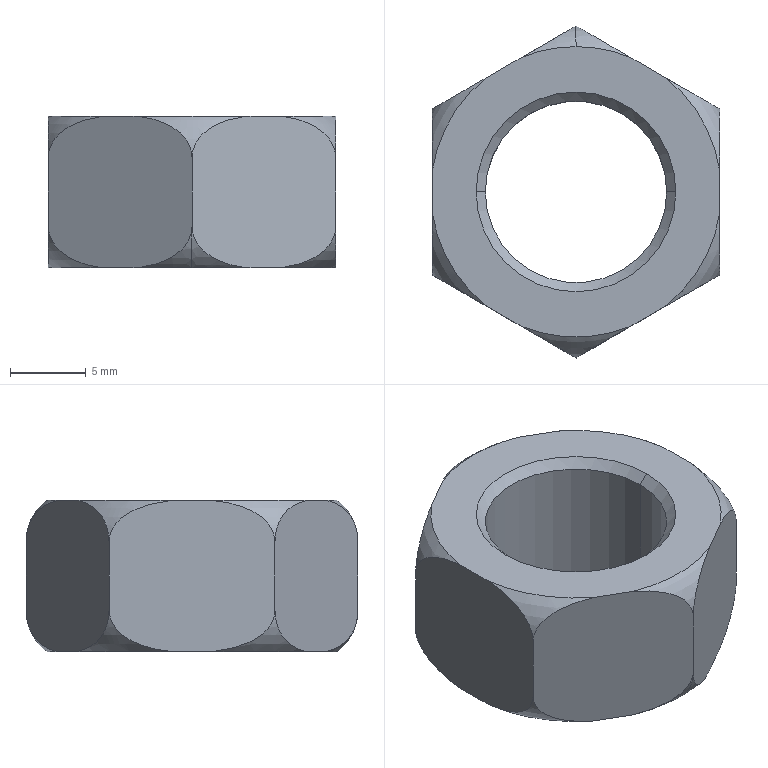Part | NX | 1 solid | 28 faces | box 19 x 21.939 x 10 mm | volume 1960 mm3 | torus 14 | plane 8 | cone 4 | cylinder 2 | commonest cylinder face diameters 12 x2
STEP:
#1=CARTESIAN_POINT('',(6.,0.,-4.4));
#2=VERTEX_POINT('',#1);
#3=CARTESIAN_POINT('',(-6.,0.,-4.4));
#4=VERTEX_POINT('',#3);
#5=CARTESIAN_POINT('',(0.,0.,-4.4));
#6=DIRECTION('',(0.,0.,1.));
#7=DIRECTION('',(-1.,0.,0.));
#8=AXIS2_PLACEMENT_3D('',#5,#6,#7);
#9=CIRCLE('',#8,6.);
#10=EDGE_CURVE('',#2,#4,#9,.T.);
#11=ORIENTED_EDGE('',*,*,#10,.T.);
#12=CARTESIAN_POINT('',(-6.6,0.,-5.));
#13=VERTEX_POINT('',#12);
#14=CARTESIAN_POINT('',(-6.3,0.,-4.7));
#15=DIRECTION('',(-0.7071,0.,-0.7071));
#16=VECTOR('',#15,1000.);
#17=LINE('',#14,#16);
#18=EDGE_CURVE('',#13,#4,#17,.F.);
#19=ORIENTED_EDGE('',*,*,#18,.F.);
#20=CARTESIAN_POINT('',(6.6,0.,-5.));
#21=VERTEX_POINT('',#20);
#22=CARTESIAN_POINT('',(0.,0.,-5.));
#23=DIRECTION('',(0.,0.,-1.));
#24=DIRECTION('',(-1.,0.,0.));
#25=AXIS2_PLACEMENT_3D('',#22,#23,#24);
#26=CIRCLE('',#25,6.6);
#27=EDGE_CURVE('',#13,#21,#26,.T.);
#28=ORIENTED_EDGE('',*,*,#27,.T.);
#29=CARTESIAN_POINT('',(6.3,0.,-4.7));
#30=DIRECTION('',(0.7071,0.,-0.7071));
#31=VECTOR('',#30,1000.);
#32=LINE('',#29,#31);
#33=EDGE_CURVE('',#21,#2,#32,.F.);
#34=ORIENTED_EDGE('',*,*,#33,.T.);
#35=EDGE_LOOP('',(#11,#19,#28,#34));
#36=FACE_BOUND('',#35,.T.);
#37=CARTESIAN_POINT('',(0.,0.,-4.7));
#38=DIRECTION('',(0.,0.,-1.));
#39=DIRECTION('',(-1.,0.,0.));
#40=AXIS2_PLACEMENT_3D('',#37,#38,#39);
#41=CONICAL_SURFACE('',#40,6.3,0.7854);
#42=ADVANCED_FACE('',(#36),#41,.F.);
#43=ORIENTED_EDGE('',*,*,#10,.F.);
#44=CARTESIAN_POINT('',(6.,0.,4.4));
#45=VERTEX_POINT('',#44);
#46=CARTESIAN_POINT('',(6.,0.,0.));
#47=DIRECTION('',(0.,0.,1.));
#48=VECTOR('',#47,1000.);
#49=LINE('',#46,#48);
#50=EDGE_CURVE('',#45,#2,#49,.F.);
#51=ORIENTED_EDGE('',*,*,#50,.F.);
#52=CARTESIAN_POINT('',(-6.,0.,4.4));
#53=VERTEX_POINT('',#52);
#54=CARTESIAN_POINT('',(0.,0.,4.4));
#55=DIRECTION('',(0.,0.,-1.));
#56=DIRECTION('',(-1.,0.,0.));
#57=AXIS2_PLACEMENT_3D('',#54,#55,#56);
#58=CIRCLE('',#57,6.);
#59=EDGE_CURVE('',#53,#45,#58,.T.);
#60=ORIENTED_EDGE('',*,*,#59,.F.);
#61=CARTESIAN_POINT('',(-6.,0.,0.));
#62=DIRECTION('',(0.,0.,1.));
#63=VECTOR('',#62,1000.);
#64=LINE('',#61,#63);
#65=EDGE_CURVE('',#53,#4,#64,.F.);
#66=ORIENTED_EDGE('',*,*,#65,.T.);
#67=EDGE_LOOP('',(#43,#51,#60,#66));
#68=FACE_BOUND('',#67,.T.);
#69=CARTESIAN_POINT('',(0.,0.,0.));
#70=DIRECTION('',(0.,0.,1.));
#71=DIRECTION('',(-1.,0.,0.));
#72=AXIS2_PLACEMENT_3D('',#69,#70,#71);
#73=CYLINDRICAL_SURFACE('',#72,6.);
#74=ADVANCED_FACE('',(#68),#73,.F.);
#75=CARTESIAN_POINT('',(5.938,7.542,-5.));
#76=VERTEX_POINT('',#75);
#77=CARTESIAN_POINT('',(9.5,1.371,-5.));
#78=VERTEX_POINT('',#77);
#79=CARTESIAN_POINT('',(0.,0.,-5.));
#80=DIRECTION('',(0.,0.,-1.));
#81=DIRECTION('',(-1.,0.,0.));
#82=AXIS2_PLACEMENT_3D('',#79,#80,#81);
#83=CIRCLE('',#82,9.598);
#84=EDGE_CURVE('',#76,#78,#83,.T.);
#85=ORIENTED_EDGE('',*,*,#84,.T.);
#86=CARTESIAN_POINT('',(9.5,-1.371,-5.));
#87=VERTEX_POINT('',#86);
#88=CARTESIAN_POINT('',(9.5,-1.371,-5.));
#89=DIRECTION('',(0.,1.,0.));
#90=VECTOR('',#89,1000.);
#91=LINE('',#88,#90);
#92=EDGE_CURVE('',#87,#78,#91,.T.);
#93=ORIENTED_EDGE('',*,*,#92,.F.);
#94=CARTESIAN_POINT('',(5.938,-7.542,-5.));
#95=VERTEX_POINT('',#94);
#96=CARTESIAN_POINT('',(0.,0.,-5.));
#97=DIRECTION('',(0.,0.,-1.));
#98=DIRECTION('',(-1.,0.,0.));
#99=AXIS2_PLACEMENT_3D('',#96,#97,#98);
#100=CIRCLE('',#99,9.598);
#101=EDGE_CURVE('',#87,#95,#100,.T.);
#102=ORIENTED_EDGE('',*,*,#101,.T.);
#103=CARTESIAN_POINT('',(3.562,-8.913,-5.));
#104=VERTEX_POINT('',#103);
#105=CARTESIAN_POINT('',(3.562,-8.913,-5.));
#106=DIRECTION('',(0.866,0.5,0.));
#107=VECTOR('',#106,1000.);
#108=LINE('',#105,#107);
#109=EDGE_CURVE('',#104,#95,#108,.T.);
#110=ORIENTED_EDGE('',*,*,#109,.F.);
#111=CARTESIAN_POINT('',(0.,-9.598,-5.));
#112=VERTEX_POINT('',#111);
#113=CARTESIAN_POINT('',(0.,0.,-5.));
#114=DIRECTION('',(0.,0.,-1.));
#115=DIRECTION('',(-1.,0.,0.));
#116=AXIS2_PLACEMENT_3D('',#113,#114,#115);
#117=CIRCLE('',#116,9.598);
#118=EDGE_CURVE('',#104,#112,#117,.T.);
#119=ORIENTED_EDGE('',*,*,#118,.T.);
#120=CARTESIAN_POINT('',(-3.562,-8.913,-5.));
#121=VERTEX_POINT('',#120);
#122=CARTESIAN_POINT('',(0.,0.,-5.));
#123=DIRECTION('',(0.,0.,-1.));
#124=DIRECTION('',(-1.,0.,0.));
#125=AXIS2_PLACEMENT_3D('',#122,#123,#124);
#126=CIRCLE('',#125,9.598);
#127=EDGE_CURVE('',#112,#121,#126,.T.);
#128=ORIENTED_EDGE('',*,*,#127,.T.);
#129=CARTESIAN_POINT('',(-5.938,-7.542,-5.));
#130=VERTEX_POINT('',#129);
#131=CARTESIAN_POINT('',(-5.938,-7.542,-5.));
#132=DIRECTION('',(0.866,-0.5,0.));
#133=VECTOR('',#132,1000.);
#134=LINE('',#131,#133);
#135=EDGE_CURVE('',#130,#121,#134,.T.);
#136=ORIENTED_EDGE('',*,*,#135,.F.);
#137=CARTESIAN_POINT('',(-9.5,-1.371,-5.));
#138=VERTEX_POINT('',#137);
#139=CARTESIAN_POINT('',(0.,0.,-5.));
#140=DIRECTION('',(0.,0.,-1.));
#141=DIRECTION('',(-1.,0.,0.));
#142=AXIS2_PLACEMENT_3D('',#139,#140,#141);
#143=CIRCLE('',#142,9.598);
#144=EDGE_CURVE('',#130,#138,#143,.T.);
#145=ORIENTED_EDGE('',*,*,#144,.T.);
#146=CARTESIAN_POINT('',(-9.5,1.371,-5.));
#147=VERTEX_POINT('',#146);
#148=CARTESIAN_POINT('',(-9.5,1.371,-5.));
#149=DIRECTION('',(0.,-1.,0.));
#150=VECTOR('',#149,1000.);
#151=LINE('',#148,#150);
#152=EDGE_CURVE('',#147,#138,#151,.T.);
#153=ORIENTED_EDGE('',*,*,#152,.F.);
#154=CARTESIAN_POINT('',(-5.938,7.542,-5.));
#155=VERTEX_POINT('',#154);
#156=CARTESIAN_POINT('',(0.,0.,-5.));
#157=DIRECTION('',(0.,0.,-1.));
#158=DIRECTION('',(-1.,0.,0.));
#159=AXIS2_PLACEMENT_3D('',#156,#157,#158);
#160=CIRCLE('',#159,9.598);
#161=EDGE_CURVE('',#147,#155,#160,.T.);
#162=ORIENTED_EDGE('',*,*,#161,.T.);
#163=CARTESIAN_POINT('',(-3.562,8.913,-5.));
#164=VERTEX_POINT('',#163);
#165=CARTESIAN_POINT('',(-3.562,8.913,-5.));
#166=DIRECTION('',(-0.866,-0.5,0.));
#167=VECTOR('',#166,1000.);
#168=LINE('',#165,#167);
#169=EDGE_CURVE('',#164,#155,#168,.T.);
#170=ORIENTED_EDGE('',*,*,#169,.F.);
#171=CARTESIAN_POINT('',(3.562,8.913,-5.));
#172=VERTEX_POINT('',#171);
#173=CARTESIAN_POINT('',(0.,0.,-5.));
#174=DIRECTION('',(0.,0.,-1.));
#175=DIRECTION('',(-1.,0.,0.));
#176=AXIS2_PLACEMENT_3D('',#173,#174,#175);
#177=CIRCLE('',#176,9.598);
#178=EDGE_CURVE('',#164,#172,#177,.T.);
#179=ORIENTED_EDGE('',*,*,#178,.T.);
#180=CARTESIAN_POINT('',(5.938,7.542,-5.));
#181=DIRECTION('',(-0.866,0.5,0.));
#182=VECTOR('',#181,1000.);
#183=LINE('',#180,#182);
#184=EDGE_CURVE('',#76,#172,#183,.T.);
#185=ORIENTED_EDGE('',*,*,#184,.F.);
#186=EDGE_LOOP('',(#85,#93,#102,#110,#119,#128,#136,#145,#153,#162,#170,#179,#185));
#187=FACE_BOUND('',#186,.T.);
#188=CARTESIAN_POINT('',(0.,0.,-5.));
#189=DIRECTION('',(0.,0.,-1.));
#190=DIRECTION('',(-1.,0.,0.));
#191=AXIS2_PLACEMENT_3D('',#188,#189,#190);
#192=CIRCLE('',#191,6.6);
#193=EDGE_CURVE('',#21,#13,#192,.T.);
#194=ORIENTED_EDGE('',*,*,#193,.F.);
#195=ORIENTED_EDGE('',*,*,#27,.F.);
#196=EDGE_LOOP('',(#194,#195));
#197=FACE_BOUND('',#196,.T.);
#198=CARTESIAN_POINT('',(0.,0.,-5.));
#199=DIRECTION('',(0.,0.,1.));
#200=DIRECTION('',(1.,0.,0.));
#201=AXIS2_PLACEMENT_3D('',#198,#199,#200);
#202=PLANE('',#201);
#203=ADVANCED_FACE('',(#187,#197),#202,.F.);
#204=CARTESIAN_POINT('',(-6.6,0.,5.));
#205=VERTEX_POINT('',#204);
#206=CARTESIAN_POINT('',(6.6,0.,5.));
#207=VERTEX_POINT('',#206);
#208=CARTESIAN_POINT('',(0.,0.,5.));
#209=DIRECTION('',(0.,0.,1.));
#210=DIRECTION('',(-1.,0.,0.));
#211=AXIS2_PLACEMENT_3D('',#208,#209,#210);
#212=CIRCLE('',#211,6.6);
#213=EDGE_CURVE('',#205,#207,#212,.T.);
#214=ORIENTED_EDGE('',*,*,#213,.T.);
#215=CARTESIAN_POINT('',(6.3,0.,4.7));
#216=DIRECTION('',(0.7071,0.,0.7071));
#217=VECTOR('',#216,1000.);
#218=LINE('',#215,#217);
#219=EDGE_CURVE('',#45,#207,#218,.T.);
#220=ORIENTED_EDGE('',*,*,#219,.F.);
#221=CARTESIAN_POINT('',(0.,0.,4.4));
#222=DIRECTION('',(0.,0.,-1.));
#223=DIRECTION('',(-1.,0.,0.));
#224=AXIS2_PLACEMENT_3D('',#221,#222,#223);
#225=CIRCLE('',#224,6.);
#226=EDGE_CURVE('',#45,#53,#225,.T.);
#227=ORIENTED_EDGE('',*,*,#226,.T.);
#228=CARTESIAN_POINT('',(-6.3,0.,4.7));
#229=DIRECTION('',(-0.7071,0.,0.7071));
#230=VECTOR('',#229,1000.);
#231=LINE('',#228,#230);
#232=EDGE_CURVE('',#53,#205,#231,.T.);
#233=ORIENTED_EDGE('',*,*,#232,.T.);
#234=EDGE_LOOP('',(#214,#220,#227,#233));
#235=FACE_BOUND('',#234,.T.);
#236=CARTESIAN_POINT('',(0.,0.,4.7));
#237=DIRECTION('',(0.,0.,1.));
#238=DIRECTION('',(1.,0.,0.));
#239=AXIS2_PLACEMENT_3D('',#236,#237,#238);
#240=CONICAL_SURFACE('',#239,6.3,0.7854);
#241=ADVANCED_FACE('',(#235),#240,.F.);
#242=CARTESIAN_POINT('',(9.5,1.371,5.));
#243=VERTEX_POINT('',#242);
#244=CARTESIAN_POINT('',(5.938,7.542,5.));
#245=VERTEX_POINT('',#244);
#246=CARTESIAN_POINT('',(0.,0.,5.));
#247=DIRECTION('',(0.,0.,1.));
#248=DIRECTION('',(1.,0.,0.));
#249=AXIS2_PLACEMENT_3D('',#246,#247,#248);
#250=CIRCLE('',#249,9.598);
#251=EDGE_CURVE('',#243,#245,#250,.T.);
#252=ORIENTED_EDGE('',*,*,#251,.T.);
#253=CARTESIAN_POINT('',(3.562,8.913,5.));
#254=VERTEX_POINT('',#253);
#255=CARTESIAN_POINT('',(3.562,8.913,5.));
#256=DIRECTION('',(0.866,-0.5,0.));
#257=VECTOR('',#256,1000.);
#258=LINE('',#255,#257);
#259=EDGE_CURVE('',#254,#245,#258,.T.);
#260=ORIENTED_EDGE('',*,*,#259,.F.);
#261=CARTESIAN_POINT('',(0.,9.598,5.));
#262=VERTEX_POINT('',#261);
#263=CARTESIAN_POINT('',(0.,0.,5.));
#264=DIRECTION('',(0.,0.,1.));
#265=DIRECTION('',(1.,0.,0.));
#266=AXIS2_PLACEMENT_3D('',#263,#264,#265);
#267=CIRCLE('',#266,9.598);
#268=EDGE_CURVE('',#254,#262,#267,.T.);
#269=ORIENTED_EDGE('',*,*,#268,.T.);
#270=CARTESIAN_POINT('',(-3.562,8.913,5.));
#271=VERTEX_POINT('',#270);
#272=CARTESIAN_POINT('',(0.,0.,5.));
#273=DIRECTION('',(0.,0.,1.));
#274=DIRECTION('',(1.,0.,0.));
#275=AXIS2_PLACEMENT_3D('',#272,#273,#274);
#276=CIRCLE('',#275,9.598);
#277=EDGE_CURVE('',#262,#271,#276,.T.);
#278=ORIENTED_EDGE('',*,*,#277,.T.);
#279=CARTESIAN_POINT('',(-5.938,7.542,5.));
#280=VERTEX_POINT('',#279);
#281=CARTESIAN_POINT('',(-5.938,7.542,5.));
#282=DIRECTION('',(0.866,0.5,0.));
#283=VECTOR('',#282,1000.);
#284=LINE('',#281,#283);
#285=EDGE_CURVE('',#280,#271,#284,.T.);
#286=ORIENTED_EDGE('',*,*,#285,.F.);
#287=CARTESIAN_POINT('',(-9.5,1.371,5.));
#288=VERTEX_POINT('',#287);
#289=CARTESIAN_POINT('',(0.,0.,5.));
#290=DIRECTION('',(0.,0.,1.));
#291=DIRECTION('',(1.,0.,0.));
#292=AXIS2_PLACEMENT_3D('',#289,#290,#291);
#293=CIRCLE('',#292,9.598);
#294=EDGE_CURVE('',#280,#288,#293,.T.);
#295=ORIENTED_EDGE('',*,*,#294,.T.);
#296=CARTESIAN_POINT('',(-9.5,-1.371,5.));
#297=VERTEX_POINT('',#296);
#298=CARTESIAN_POINT('',(-9.5,-1.371,5.));
#299=DIRECTION('',(0.,1.,0.));
#300=VECTOR('',#299,1000.);
#301=LINE('',#298,#300);
#302=EDGE_CURVE('',#297,#288,#301,.T.);
#303=ORIENTED_EDGE('',*,*,#302,.F.);
#304=CARTESIAN_POINT('',(-5.938,-7.542,5.));
#305=VERTEX_POINT('',#304);
#306=CARTESIAN_POINT('',(0.,0.,5.));
#307=DIRECTION('',(0.,0.,1.));
#308=DIRECTION('',(1.,0.,0.));
#309=AXIS2_PLACEMENT_3D('',#306,#307,#308);
#310=CIRCLE('',#309,9.598);
#311=EDGE_CURVE('',#297,#305,#310,.T.);
#312=ORIENTED_EDGE('',*,*,#311,.T.);
#313=CARTESIAN_POINT('',(-3.562,-8.913,5.));
#314=VERTEX_POINT('',#313);
#315=CARTESIAN_POINT('',(-3.562,-8.913,5.));
#316=DIRECTION('',(-0.866,0.5,0.));
#317=VECTOR('',#316,1000.);
#318=LINE('',#315,#317);
#319=EDGE_CURVE('',#314,#305,#318,.T.);
#320=ORIENTED_EDGE('',*,*,#319,.F.);
#321=CARTESIAN_POINT('',(3.562,-8.913,5.));
#322=VERTEX_POINT('',#321);
#323=CARTESIAN_POINT('',(0.,0.,5.));
#324=DIRECTION('',(0.,0.,1.));
#325=DIRECTION('',(1.,0.,0.));
#326=AXIS2_PLACEMENT_3D('',#323,#324,#325);
#327=CIRCLE('',#326,9.598);
#328=EDGE_CURVE('',#314,#322,#327,.T.);
#329=ORIENTED_EDGE('',*,*,#328,.T.);
#330=CARTESIAN_POINT('',(5.938,-7.542,5.));
#331=VERTEX_POINT('',#330);
#332=CARTESIAN_POINT('',(5.938,-7.542,5.));
#333=DIRECTION('',(-0.866,-0.5,0.));
#334=VECTOR('',#333,1000.);
#335=LINE('',#332,#334);
#336=EDGE_CURVE('',#331,#322,#335,.T.);
#337=ORIENTED_EDGE('',*,*,#336,.F.);
#338=CARTESIAN_POINT('',(9.5,-1.371,5.));
#339=VERTEX_POINT('',#338);
#340=CARTESIAN_POINT('',(0.,0.,5.));
#341=DIRECTION('',(0.,0.,1.));
#342=DIRECTION('',(1.,0.,0.));
#343=AXIS2_PLACEMENT_3D('',#340,#341,#342);
#344=CIRCLE('',#343,9.598);
#345=EDGE_CURVE('',#331,#339,#344,.T.);
#346=ORIENTED_EDGE('',*,*,#345,.T.);
#347=CARTESIAN_POINT('',(9.5,1.371,5.));
#348=DIRECTION('',(0.,-1.,0.));
#349=VECTOR('',#348,1000.);
#350=LINE('',#347,#349);
#351=EDGE_CURVE('',#243,#339,#350,.T.);
#352=ORIENTED_EDGE('',*,*,#351,.F.);
#353=EDGE_LOOP('',(#252,#260,#269,#278,#286,#295,#303,#312,#320,#329,#337,#346,#352));
#354=FACE_BOUND('',#353,.T.);
#355=ORIENTED_EDGE('',*,*,#213,.F.);
#356=CARTESIAN_POINT('',(0.,0.,5.));
#357=DIRECTION('',(0.,0.,1.));
#358=DIRECTION('',(-1.,0.,0.));
#359=AXIS2_PLACEMENT_3D('',#356,#357,#358);
#360=CIRCLE('',#359,6.6);
#361=EDGE_CURVE('',#207,#205,#360,.T.);
#362=ORIENTED_EDGE('',*,*,#361,.F.);
#363=EDGE_LOOP('',(#355,#362));
#364=FACE_BOUND('',#363,.T.);
#365=CARTESIAN_POINT('',(0.,0.,5.));
#366=DIRECTION('',(0.,0.,1.));
#367=DIRECTION('',(1.,0.,0.));
#368=AXIS2_PLACEMENT_3D('',#365,#366,#367);
#369=PLANE('',#368);
#370=ADVANCED_FACE('',(#354,#364),#369,.T.);
#371=CARTESIAN_POINT('',(-9.5,5.485,-2.258));
#372=VERTEX_POINT('',#371);
#373=CARTESIAN_POINT('',(-5.938,7.542,-5.));
#374=CARTESIAN_POINT('',(-6.359,7.298,-4.948));
#375=CARTESIAN_POINT('',(-6.904,6.984,-4.844));
#376=CARTESIAN_POINT('',(-7.693,6.528,-4.564));
#377=CARTESIAN_POINT('',(-8.328,6.161,-4.245));
#378=CARTESIAN_POINT('',(-9.176,5.672,-3.582));
#379=CARTESIAN_POINT('',(-9.5,5.485,-2.693));
#380=CARTESIAN_POINT('',(-9.5,5.485,-2.258));
#381=B_SPLINE_CURVE_WITH_KNOTS('',3,(#373,#374,#375,#376,#377,#378,#379,#380),.UNSPECIFIED.,.F.,.F.,(4,1,1,1,1,4),(0.,0.25,0.375,0.5,0.75,1.),.UNSPECIFIED.);
#382=EDGE_CURVE('',#155,#372,#381,.T.);
#383=ORIENTED_EDGE('',*,*,#382,.F.);
#384=ORIENTED_EDGE('',*,*,#161,.F.);
#385=CARTESIAN_POINT('',(-9.5,5.485,-2.258));
#386=CARTESIAN_POINT('',(-9.5,5.485,-2.477));
#387=CARTESIAN_POINT('',(-9.5,5.416,-2.892));
#388=CARTESIAN_POINT('',(-9.5,5.011,-3.534));
#389=CARTESIAN_POINT('',(-9.5,4.593,-3.928));
#390=CARTESIAN_POINT('',(-9.5,3.922,-4.343));
#391=CARTESIAN_POINT('',(-9.5,3.431,-4.548));
#392=CARTESIAN_POINT('',(-9.5,2.599,-4.82));
#393=CARTESIAN_POINT('',(-9.5,1.892,-4.944));
#394=CARTESIAN_POINT('',(-9.5,1.371,-5.));
#395=B_SPLINE_CURVE_WITH_KNOTS('',3,(#385,#386,#387,#388,#389,#390,#391,#392,#393,#394),.UNSPECIFIED.,.F.,.F.,(4,1,1,1,1,1,1,4),(0.,0.125,0.25,0.375,0.5,0.625,0.75,1.),.UNSPECIFIED.);
#396=EDGE_CURVE('',#372,#147,#395,.T.);
#397=ORIENTED_EDGE('',*,*,#396,.F.);
#398=EDGE_LOOP('',(#383,#384,#397));
#399=FACE_BOUND('',#398,.T.);
#400=CARTESIAN_POINT('',(0.,0.,-2.258));
#401=DIRECTION('',(0.,0.,1.));
#402=DIRECTION('',(0.,1.,0.));
#403=AXIS2_PLACEMENT_3D('',#400,#401,#402);
#404=TOROIDAL_SURFACE('',#403,7.542,3.428);
#405=ADVANCED_FACE('',(#399),#404,.T.);
#406=CARTESIAN_POINT('',(-9.5,-5.485,-2.258));
#407=VERTEX_POINT('',#406);
#408=CARTESIAN_POINT('',(-9.5,-1.371,-5.));
#409=CARTESIAN_POINT('',(-9.5,-1.858,-4.948));
#410=CARTESIAN_POINT('',(-9.5,-2.487,-4.844));
#411=CARTESIAN_POINT('',(-9.5,-3.398,-4.564));
#412=CARTESIAN_POINT('',(-9.5,-4.132,-4.245));
#413=CARTESIAN_POINT('',(-9.5,-5.111,-3.582));
#414=CARTESIAN_POINT('',(-9.5,-5.485,-2.693));
#415=CARTESIAN_POINT('',(-9.5,-5.485,-2.258));
#416=B_SPLINE_CURVE_WITH_KNOTS('',3,(#408,#409,#410,#411,#412,#413,#414,#415),.UNSPECIFIED.,.F.,.F.,(4,1,1,1,1,4),(0.,0.25,0.375,0.5,0.75,1.),.UNSPECIFIED.);
#417=EDGE_CURVE('',#138,#407,#416,.T.);
#418=ORIENTED_EDGE('',*,*,#417,.F.);
#419=ORIENTED_EDGE('',*,*,#144,.F.);
#420=CARTESIAN_POINT('',(-9.5,-5.485,-2.258));
#421=CARTESIAN_POINT('',(-9.5,-5.485,-2.477));
#422=CARTESIAN_POINT('',(-9.441,-5.519,-2.892));
#423=CARTESIAN_POINT('',(-9.089,-5.722,-3.534));
#424=CARTESIAN_POINT('',(-8.727,-5.931,-3.928));
#425=CARTESIAN_POINT('',(-8.146,-6.266,-4.343));
#426=CARTESIAN_POINT('',(-7.721,-6.512,-4.548));
#427=CARTESIAN_POINT('',(-7.,-6.928,-4.82));
#428=CARTESIAN_POINT('',(-6.388,-7.281,-4.944));
#429=CARTESIAN_POINT('',(-5.938,-7.542,-5.));
#430=B_SPLINE_CURVE_WITH_KNOTS('',3,(#420,#421,#422,#423,#424,#425,#426,#427,#428,#429),.UNSPECIFIED.,.F.,.F.,(4,1,1,1,1,1,1,4),(0.,0.125,0.25,0.375,0.5,0.625,0.75,1.),.UNSPECIFIED.);
#431=EDGE_CURVE('',#407,#130,#430,.T.);
#432=ORIENTED_EDGE('',*,*,#431,.F.);
#433=EDGE_LOOP('',(#418,#419,#432));
#434=FACE_BOUND('',#433,.T.);
#435=CARTESIAN_POINT('',(0.,0.,-2.258));
#436=DIRECTION('',(0.,0.,1.));
#437=DIRECTION('',(0.,1.,0.));
#438=AXIS2_PLACEMENT_3D('',#435,#436,#437);
#439=TOROIDAL_SURFACE('',#438,7.542,3.428);
#440=ADVANCED_FACE('',(#434),#439,.T.);
#441=CARTESIAN_POINT('',(0.,-10.97,-2.258));
#442=VERTEX_POINT('',#441);
#443=CARTESIAN_POINT('',(0.,-7.542,-2.258));
#444=DIRECTION('',(1.,0.,0.));
#445=DIRECTION('',(0.,0.,-1.));
#446=AXIS2_PLACEMENT_3D('',#443,#444,#445);
#447=CIRCLE('',#446,3.428);
#448=EDGE_CURVE('',#442,#112,#447,.T.);
#449=ORIENTED_EDGE('',*,*,#448,.F.);
#450=CARTESIAN_POINT('',(-3.562,-8.913,-5.));
#451=CARTESIAN_POINT('',(-3.141,-9.156,-4.948));
#452=CARTESIAN_POINT('',(-2.596,-9.471,-4.844));
#453=CARTESIAN_POINT('',(-1.807,-9.926,-4.564));
#454=CARTESIAN_POINT('',(-1.172,-10.293,-4.245));
#455=CARTESIAN_POINT('',(-0.3236,-10.783,-3.582));
#456=CARTESIAN_POINT('',(0.,-10.97,-2.693));
#457=CARTESIAN_POINT('',(0.,-10.97,-2.258));
#458=B_SPLINE_CURVE_WITH_KNOTS('',3,(#450,#451,#452,#453,#454,#455,#456,#457),.UNSPECIFIED.,.F.,.F.,(4,1,1,1,1,4),(0.,0.25,0.375,0.5,0.75,1.),.UNSPECIFIED.);
#459=EDGE_CURVE('',#121,#442,#458,.T.);
#460=ORIENTED_EDGE('',*,*,#459,.F.);
#461=ORIENTED_EDGE('',*,*,#127,.F.);
#462=EDGE_LOOP('',(#449,#460,#461));
#463=FACE_BOUND('',#462,.T.);
#464=CARTESIAN_POINT('',(0.,0.,-2.258));
#465=DIRECTION('',(0.,0.,-1.));
#466=DIRECTION('',(0.,-1.,0.));
#467=AXIS2_PLACEMENT_3D('',#464,#465,#466);
#468=TOROIDAL_SURFACE('',#467,7.542,3.428);
#469=ADVANCED_FACE('',(#463),#468,.T.);
#470=CARTESIAN_POINT('',(0.,10.97,-2.258));
#471=VERTEX_POINT('',#470);
#472=CARTESIAN_POINT('',(3.562,8.913,-5.));
#473=CARTESIAN_POINT('',(3.141,9.156,-4.948));
#474=CARTESIAN_POINT('',(2.596,9.471,-4.844));
#475=CARTESIAN_POINT('',(1.807,9.926,-4.564));
#476=CARTESIAN_POINT('',(1.172,10.293,-4.245));
#477=CARTESIAN_POINT('',(0.3236,10.783,-3.582));
#478=CARTESIAN_POINT('',(0.,10.97,-2.693));
#479=CARTESIAN_POINT('',(0.,10.97,-2.258));
#480=B_SPLINE_CURVE_WITH_KNOTS('',3,(#472,#473,#474,#475,#476,#477,#478,#479),.UNSPECIFIED.,.F.,.F.,(4,1,1,1,1,4),(0.,0.25,0.375,0.5,0.75,1.),.UNSPECIFIED.);
#481=EDGE_CURVE('',#172,#471,#480,.T.);
#482=ORIENTED_EDGE('',*,*,#481,.F.);
#483=ORIENTED_EDGE('',*,*,#178,.F.);
#484=CARTESIAN_POINT('',(0.,10.97,-2.258));
#485=CARTESIAN_POINT('',(0.,10.97,-2.477));
#486=CARTESIAN_POINT('',(-0.05943,10.935,-2.892));
#487=CARTESIAN_POINT('',(-0.4107,10.733,-3.534));
#488=CARTESIAN_POINT('',(-0.7725,10.524,-3.928));
#489=CARTESIAN_POINT('',(-1.354,10.188,-4.343));
#490=CARTESIAN_POINT('',(-1.779,9.943,-4.548));
#491=CARTESIAN_POINT('',(-2.5,9.527,-4.82));
#492=CARTESIAN_POINT('',(-3.112,9.173,-4.944));
#493=CARTESIAN_POINT('',(-3.562,8.913,-5.));
#494=B_SPLINE_CURVE_WITH_KNOTS('',3,(#484,#485,#486,#487,#488,#489,#490,#491,#492,#493),.UNSPECIFIED.,.F.,.F.,(4,1,1,1,1,1,1,4),(0.,0.125,0.25,0.375,0.5,0.625,0.75,1.),.UNSPECIFIED.);
#495=EDGE_CURVE('',#471,#164,#494,.T.);
#496=ORIENTED_EDGE('',*,*,#495,.F.);
#497=EDGE_LOOP('',(#482,#483,#496));
#498=FACE_BOUND('',#497,.T.);
#499=CARTESIAN_POINT('',(0.,0.,-2.258));
#500=DIRECTION('',(0.,0.,-1.));
#501=DIRECTION('',(0.,-1.,0.));
#502=AXIS2_PLACEMENT_3D('',#499,#500,#501);
#503=TOROIDAL_SURFACE('',#502,7.542,3.428);
#504=ADVANCED_FACE('',(#498),#503,.T.);
#505=CARTESIAN_POINT('',(9.5,-5.485,-2.258));
#506=VERTEX_POINT('',#505);
#507=CARTESIAN_POINT('',(5.938,-7.542,-5.));
#508=CARTESIAN_POINT('',(6.359,-7.298,-4.948));
#509=CARTESIAN_POINT('',(6.904,-6.984,-4.844));
#510=CARTESIAN_POINT('',(7.693,-6.528,-4.564));
#511=CARTESIAN_POINT('',(8.328,-6.161,-4.245));
#512=CARTESIAN_POINT('',(9.176,-5.672,-3.582));
#513=CARTESIAN_POINT('',(9.5,-5.485,-2.693));
#514=CARTESIAN_POINT('',(9.5,-5.485,-2.258));
#515=B_SPLINE_CURVE_WITH_KNOTS('',3,(#507,#508,#509,#510,#511,#512,#513,#514),.UNSPECIFIED.,.F.,.F.,(4,1,1,1,1,4),(0.,0.25,0.375,0.5,0.75,1.),.UNSPECIFIED.);
#516=EDGE_CURVE('',#95,#506,#515,.T.);
#517=ORIENTED_EDGE('',*,*,#516,.F.);
#518=ORIENTED_EDGE('',*,*,#101,.F.);
#519=CARTESIAN_POINT('',(9.5,-5.485,-2.258));
#520=CARTESIAN_POINT('',(9.5,-5.485,-2.477));
#521=CARTESIAN_POINT('',(9.5,-5.416,-2.892));
#522=CARTESIAN_POINT('',(9.5,-5.011,-3.534));
#523=CARTESIAN_POINT('',(9.5,-4.593,-3.928));
#524=CARTESIAN_POINT('',(9.5,-3.922,-4.343));
#525=CARTESIAN_POINT('',(9.5,-3.431,-4.548));
#526=CARTESIAN_POINT('',(9.5,-2.599,-4.82));
#527=CARTESIAN_POINT('',(9.5,-1.892,-4.944));
#528=CARTESIAN_POINT('',(9.5,-1.371,-5.));
#529=B_SPLINE_CURVE_WITH_KNOTS('',3,(#519,#520,#521,#522,#523,#524,#525,#526,#527,#528),.UNSPECIFIED.,.F.,.F.,(4,1,1,1,1,1,1,4),(0.,0.125,0.25,0.375,0.5,0.625,0.75,1.),.UNSPECIFIED.);
#530=EDGE_CURVE('',#506,#87,#529,.T.);
#531=ORIENTED_EDGE('',*,*,#530,.F.);
#532=EDGE_LOOP('',(#517,#518,#531));
#533=FACE_BOUND('',#532,.T.);
#534=CARTESIAN_POINT('',(0.,0.,-2.258));
#535=DIRECTION('',(0.,0.,1.));
#536=DIRECTION('',(0.,1.,0.));
#537=AXIS2_PLACEMENT_3D('',#534,#535,#536);
#538=TOROIDAL_SURFACE('',#537,7.542,3.428);
#539=ADVANCED_FACE('',(#533),#538,.T.);
#540=CARTESIAN_POINT('',(9.5,5.485,-2.258));
#541=VERTEX_POINT('',#540);
#542=CARTESIAN_POINT('',(9.5,1.371,-5.));
#543=CARTESIAN_POINT('',(9.5,1.858,-4.948));
#544=CARTESIAN_POINT('',(9.5,2.487,-4.844));
#545=CARTESIAN_POINT('',(9.5,3.398,-4.564));
#546=CARTESIAN_POINT('',(9.5,4.132,-4.245));
#547=CARTESIAN_POINT('',(9.5,5.111,-3.582));
#548=CARTESIAN_POINT('',(9.5,5.485,-2.693));
#549=CARTESIAN_POINT('',(9.5,5.485,-2.258));
#550=B_SPLINE_CURVE_WITH_KNOTS('',3,(#542,#543,#544,#545,#546,#547,#548,#549),.UNSPECIFIED.,.F.,.F.,(4,1,1,1,1,4),(0.,0.25,0.375,0.5,0.75,1.),.UNSPECIFIED.);
#551=EDGE_CURVE('',#78,#541,#550,.T.);
#552=ORIENTED_EDGE('',*,*,#551,.F.);
#553=ORIENTED_EDGE('',*,*,#84,.F.);
#554=CARTESIAN_POINT('',(9.5,5.485,-2.258));
#555=CARTESIAN_POINT('',(9.5,5.485,-2.477));
#556=CARTESIAN_POINT('',(9.441,5.519,-2.892));
#557=CARTESIAN_POINT('',(9.089,5.722,-3.534));
#558=CARTESIAN_POINT('',(8.727,5.931,-3.928));
#559=CARTESIAN_POINT('',(8.146,6.266,-4.343));
#560=CARTESIAN_POINT('',(7.721,6.512,-4.548));
#561=CARTESIAN_POINT('',(7.,6.928,-4.82));
#562=CARTESIAN_POINT('',(6.388,7.281,-4.944));
#563=CARTESIAN_POINT('',(5.938,7.542,-5.));
#564=B_SPLINE_CURVE_WITH_KNOTS('',3,(#554,#555,#556,#557,#558,#559,#560,#561,#562,#563),.UNSPECIFIED.,.F.,.F.,(4,1,1,1,1,1,1,4),(0.,0.125,0.25,0.375,0.5,0.625,0.75,1.),.UNSPECIFIED.);
#565=EDGE_CURVE('',#541,#76,#564,.T.);
#566=ORIENTED_EDGE('',*,*,#565,.F.);
#567=EDGE_LOOP('',(#552,#553,#566));
#568=FACE_BOUND('',#567,.T.);
#569=CARTESIAN_POINT('',(0.,0.,-2.258));
#570=DIRECTION('',(0.,0.,1.));
#571=DIRECTION('',(0.,1.,0.));
#572=AXIS2_PLACEMENT_3D('',#569,#570,#571);
#573=TOROIDAL_SURFACE('',#572,7.542,3.428);
#574=ADVANCED_FACE('',(#568),#573,.T.);
#575=ORIENTED_EDGE('',*,*,#551,.T.);
#576=CARTESIAN_POINT('',(9.5,5.485,2.258));
#577=VERTEX_POINT('',#576);
#578=CARTESIAN_POINT('',(9.5,5.485,2.258));
#579=DIRECTION('',(0.,0.,-1.));
#580=VECTOR('',#579,1000.);
#581=LINE('',#578,#580);
#582=EDGE_CURVE('',#577,#541,#581,.T.);
#583=ORIENTED_EDGE('',*,*,#582,.F.);
#584=CARTESIAN_POINT('',(9.5,5.485,2.258));
#585=CARTESIAN_POINT('',(9.5,5.485,2.477));
#586=CARTESIAN_POINT('',(9.5,5.416,2.892));
#587=CARTESIAN_POINT('',(9.5,5.011,3.534));
#588=CARTESIAN_POINT('',(9.5,4.593,3.928));
#589=CARTESIAN_POINT('',(9.5,3.922,4.343));
#590=CARTESIAN_POINT('',(9.5,3.431,4.548));
#591=CARTESIAN_POINT('',(9.5,2.599,4.82));
#592=CARTESIAN_POINT('',(9.5,1.892,4.944));
#593=CARTESIAN_POINT('',(9.5,1.371,5.));
#594=B_SPLINE_CURVE_WITH_KNOTS('',3,(#584,#585,#586,#587,#588,#589,#590,#591,#592,#593),.UNSPECIFIED.,.F.,.F.,(4,1,1,1,1,1,1,4),(0.,0.125,0.25,0.375,0.5,0.625,0.75,1.),.UNSPECIFIED.);
#595=EDGE_CURVE('',#577,#243,#594,.T.);
#596=ORIENTED_EDGE('',*,*,#595,.T.);
#597=ORIENTED_EDGE('',*,*,#351,.T.);
#598=CARTESIAN_POINT('',(9.5,-5.485,2.258));
#599=VERTEX_POINT('',#598);
#600=CARTESIAN_POINT('',(9.5,-1.371,5.));
#601=CARTESIAN_POINT('',(9.5,-1.858,4.948));
#602=CARTESIAN_POINT('',(9.5,-2.487,4.844));
#603=CARTESIAN_POINT('',(9.5,-3.398,4.564));
#604=CARTESIAN_POINT('',(9.5,-4.132,4.245));
#605=CARTESIAN_POINT('',(9.5,-5.111,3.582));
#606=CARTESIAN_POINT('',(9.5,-5.485,2.693));
#607=CARTESIAN_POINT('',(9.5,-5.485,2.258));
#608=B_SPLINE_CURVE_WITH_KNOTS('',3,(#600,#601,#602,#603,#604,#605,#606,#607),.UNSPECIFIED.,.F.,.F.,(4,1,1,1,1,4),(0.,0.25,0.375,0.5,0.75,1.),.UNSPECIFIED.);
#609=EDGE_CURVE('',#339,#599,#608,.T.);
#610=ORIENTED_EDGE('',*,*,#609,.T.);
#611=CARTESIAN_POINT('',(9.5,-5.485,2.258));
#612=DIRECTION('',(0.,0.,-1.));
#613=VECTOR('',#612,1000.);
#614=LINE('',#611,#613);
#615=EDGE_CURVE('',#599,#506,#614,.T.);
#616=ORIENTED_EDGE('',*,*,#615,.T.);
#617=ORIENTED_EDGE('',*,*,#530,.T.);
#618=ORIENTED_EDGE('',*,*,#92,.T.);
#619=EDGE_LOOP('',(#575,#583,#596,#597,#610,#616,#617,#618));
#620=FACE_BOUND('',#619,.T.);
#621=CARTESIAN_POINT('',(9.5,5.485,0.));
#622=DIRECTION('',(1.,0.,0.));
#623=DIRECTION('',(0.,1.,0.));
#624=AXIS2_PLACEMENT_3D('',#621,#622,#623);
#625=PLANE('',#624);
#626=ADVANCED_FACE('',(#620),#625,.T.);
#627=CARTESIAN_POINT('',(-9.5,5.485,2.258));
#628=VERTEX_POINT('',#627);
#629=CARTESIAN_POINT('',(-9.5,5.485,2.258));
#630=CARTESIAN_POINT('',(-9.5,5.485,2.477));
#631=CARTESIAN_POINT('',(-9.441,5.519,2.892));
#632=CARTESIAN_POINT('',(-9.089,5.722,3.534));
#633=CARTESIAN_POINT('',(-8.727,5.931,3.928));
#634=CARTESIAN_POINT('',(-8.146,6.266,4.343));
#635=CARTESIAN_POINT('',(-7.721,6.512,4.548));
#636=CARTESIAN_POINT('',(-7.,6.928,4.82));
#637=CARTESIAN_POINT('',(-6.388,7.281,4.944));
#638=CARTESIAN_POINT('',(-5.938,7.542,5.));
#639=B_SPLINE_CURVE_WITH_KNOTS('',3,(#629,#630,#631,#632,#633,#634,#635,#636,#637,#638),.UNSPECIFIED.,.F.,.F.,(4,1,1,1,1,1,1,4),(0.,0.125,0.25,0.375,0.5,0.625,0.75,1.),.UNSPECIFIED.);
#640=EDGE_CURVE('',#628,#280,#639,.T.);
#641=ORIENTED_EDGE('',*,*,#640,.F.);
#642=CARTESIAN_POINT('',(-9.5,1.371,5.));
#643=CARTESIAN_POINT('',(-9.5,1.858,4.948));
#644=CARTESIAN_POINT('',(-9.5,2.487,4.844));
#645=CARTESIAN_POINT('',(-9.5,3.398,4.564));
#646=CARTESIAN_POINT('',(-9.5,4.132,4.245));
#647=CARTESIAN_POINT('',(-9.5,5.111,3.582));
#648=CARTESIAN_POINT('',(-9.5,5.485,2.693));
#649=CARTESIAN_POINT('',(-9.5,5.485,2.258));
#650=B_SPLINE_CURVE_WITH_KNOTS('',3,(#642,#643,#644,#645,#646,#647,#648,#649),.UNSPECIFIED.,.F.,.F.,(4,1,1,1,1,4),(0.,0.25,0.375,0.5,0.75,1.),.UNSPECIFIED.);
#651=EDGE_CURVE('',#288,#628,#650,.T.);
#652=ORIENTED_EDGE('',*,*,#651,.F.);
#653=ORIENTED_EDGE('',*,*,#294,.F.);
#654=EDGE_LOOP('',(#641,#652,#653));
#655=FACE_BOUND('',#654,.T.);
#656=CARTESIAN_POINT('',(0.,0.,2.258));
#657=DIRECTION('',(0.,0.,-1.));
#658=DIRECTION('',(0.,-1.,0.));
#659=AXIS2_PLACEMENT_3D('',#656,#657,#658);
#660=TOROIDAL_SURFACE('',#659,7.542,3.428);
#661=ADVANCED_FACE('',(#655),#660,.T.);
#662=CARTESIAN_POINT('',(-9.5,-5.485,2.258));
#663=VERTEX_POINT('',#662);
#664=CARTESIAN_POINT('',(-9.5,-5.485,2.258));
#665=CARTESIAN_POINT('',(-9.5,-5.485,2.477));
#666=CARTESIAN_POINT('',(-9.5,-5.416,2.892));
#667=CARTESIAN_POINT('',(-9.5,-5.011,3.534));
#668=CARTESIAN_POINT('',(-9.5,-4.593,3.928));
#669=CARTESIAN_POINT('',(-9.5,-3.922,4.343));
#670=CARTESIAN_POINT('',(-9.5,-3.431,4.548));
#671=CARTESIAN_POINT('',(-9.5,-2.599,4.82));
#672=CARTESIAN_POINT('',(-9.5,-1.892,4.944));
#673=CARTESIAN_POINT('',(-9.5,-1.371,5.));
#674=B_SPLINE_CURVE_WITH_KNOTS('',3,(#664,#665,#666,#667,#668,#669,#670,#671,#672,#673),.UNSPECIFIED.,.F.,.F.,(4,1,1,1,1,1,1,4),(0.,0.125,0.25,0.375,0.5,0.625,0.75,1.),.UNSPECIFIED.);
#675=EDGE_CURVE('',#663,#297,#674,.T.);
#676=ORIENTED_EDGE('',*,*,#675,.F.);
#677=CARTESIAN_POINT('',(-5.938,-7.542,5.));
#678=CARTESIAN_POINT('',(-6.359,-7.298,4.948));
#679=CARTESIAN_POINT('',(-6.904,-6.984,4.844));
#680=CARTESIAN_POINT('',(-7.693,-6.528,4.564));
#681=CARTESIAN_POINT('',(-8.328,-6.161,4.245));
#682=CARTESIAN_POINT('',(-9.176,-5.672,3.582));
#683=CARTESIAN_POINT('',(-9.5,-5.485,2.693));
#684=CARTESIAN_POINT('',(-9.5,-5.485,2.258));
#685=B_SPLINE_CURVE_WITH_KNOTS('',3,(#677,#678,#679,#680,#681,#682,#683,#684),.UNSPECIFIED.,.F.,.F.,(4,1,1,1,1,4),(0.,0.25,0.375,0.5,0.75,1.),.UNSPECIFIED.);
#686=EDGE_CURVE('',#305,#663,#685,.T.);
#687=ORIENTED_EDGE('',*,*,#686,.F.);
#688=ORIENTED_EDGE('',*,*,#311,.F.);
#689=EDGE_LOOP('',(#676,#687,#688));
#690=FACE_BOUND('',#689,.T.);
#691=CARTESIAN_POINT('',(0.,0.,2.258));
#692=DIRECTION('',(0.,0.,-1.));
#693=DIRECTION('',(0.,-1.,0.));
#694=AXIS2_PLACEMENT_3D('',#691,#692,#693);
#695=TOROIDAL_SURFACE('',#694,7.542,3.428);
#696=ADVANCED_FACE('',(#690),#695,.T.);
#697=CARTESIAN_POINT('',(0.,-10.97,2.258));
#698=VERTEX_POINT('',#697);
#699=CARTESIAN_POINT('',(0.,-10.97,2.258));
#700=CARTESIAN_POINT('',(0.,-10.97,2.477));
#701=CARTESIAN_POINT('',(-0.05943,-10.935,2.892));
#702=CARTESIAN_POINT('',(-0.4107,-10.733,3.534));
#703=CARTESIAN_POINT('',(-0.7725,-10.524,3.928));
#704=CARTESIAN_POINT('',(-1.354,-10.188,4.343));
#705=CARTESIAN_POINT('',(-1.779,-9.943,4.548));
#706=CARTESIAN_POINT('',(-2.5,-9.527,4.82));
#707=CARTESIAN_POINT('',(-3.112,-9.173,4.944));
#708=CARTESIAN_POINT('',(-3.562,-8.913,5.));
#709=B_SPLINE_CURVE_WITH_KNOTS('',3,(#699,#700,#701,#702,#703,#704,#705,#706,#707,#708),.UNSPECIFIED.,.F.,.F.,(4,1,1,1,1,1,1,4),(0.,0.125,0.25,0.375,0.5,0.625,0.75,1.),.UNSPECIFIED.);
#710=EDGE_CURVE('',#698,#314,#709,.T.);
#711=ORIENTED_EDGE('',*,*,#710,.F.);
#712=CARTESIAN_POINT('',(3.562,-8.913,5.));
#713=CARTESIAN_POINT('',(3.141,-9.156,4.948));
#714=CARTESIAN_POINT('',(2.596,-9.471,4.844));
#715=CARTESIAN_POINT('',(1.807,-9.926,4.564));
#716=CARTESIAN_POINT('',(1.172,-10.293,4.245));
#717=CARTESIAN_POINT('',(0.3236,-10.783,3.582));
#718=CARTESIAN_POINT('',(0.,-10.97,2.693));
#719=CARTESIAN_POINT('',(0.,-10.97,2.258));
#720=B_SPLINE_CURVE_WITH_KNOTS('',3,(#712,#713,#714,#715,#716,#717,#718,#719),.UNSPECIFIED.,.F.,.F.,(4,1,1,1,1,4),(0.,0.25,0.375,0.5,0.75,1.),.UNSPECIFIED.);
#721=EDGE_CURVE('',#322,#698,#720,.T.);
#722=ORIENTED_EDGE('',*,*,#721,.F.);
#723=ORIENTED_EDGE('',*,*,#328,.F.);
#724=EDGE_LOOP('',(#711,#722,#723));
#725=FACE_BOUND('',#724,.T.);
#726=CARTESIAN_POINT('',(0.,0.,2.258));
#727=DIRECTION('',(0.,0.,1.));
#728=DIRECTION('',(0.,1.,0.));
#729=AXIS2_PLACEMENT_3D('',#726,#727,#728);
#730=TOROIDAL_SURFACE('',#729,7.542,3.428);
#731=ADVANCED_FACE('',(#725),#730,.T.);
#732=CARTESIAN_POINT('',(9.5,-5.485,2.258));
#733=CARTESIAN_POINT('',(9.5,-5.485,2.477));
#734=CARTESIAN_POINT('',(9.441,-5.519,2.892));
#735=CARTESIAN_POINT('',(9.089,-5.722,3.534));
#736=CARTESIAN_POINT('',(8.727,-5.931,3.928));
#737=CARTESIAN_POINT('',(8.146,-6.266,4.343));
#738=CARTESIAN_POINT('',(7.721,-6.512,4.548));
#739=CARTESIAN_POINT('',(7.,-6.928,4.82));
#740=CARTESIAN_POINT('',(6.388,-7.281,4.944));
#741=CARTESIAN_POINT('',(5.938,-7.542,5.));
#742=B_SPLINE_CURVE_WITH_KNOTS('',3,(#732,#733,#734,#735,#736,#737,#738,#739,#740,#741),.UNSPECIFIED.,.F.,.F.,(4,1,1,1,1,1,1,4),(0.,0.125,0.25,0.375,0.5,0.625,0.75,1.),.UNSPECIFIED.);
#743=EDGE_CURVE('',#599,#331,#742,.T.);
#744=ORIENTED_EDGE('',*,*,#743,.F.);
#745=ORIENTED_EDGE('',*,*,#609,.F.);
#746=ORIENTED_EDGE('',*,*,#345,.F.);
#747=EDGE_LOOP('',(#744,#745,#746));
#748=FACE_BOUND('',#747,.T.);
#749=CARTESIAN_POINT('',(0.,0.,2.258));
#750=DIRECTION('',(0.,0.,-1.));
#751=DIRECTION('',(0.,-1.,0.));
#752=AXIS2_PLACEMENT_3D('',#749,#750,#751);
#753=TOROIDAL_SURFACE('',#752,7.542,3.428);
#754=ADVANCED_FACE('',(#748),#753,.T.);
#755=CARTESIAN_POINT('',(0.,10.97,2.258));
#756=VERTEX_POINT('',#755);
#757=CARTESIAN_POINT('',(0.,7.542,2.258));
#758=DIRECTION('',(1.,0.,0.));
#759=DIRECTION('',(0.,0.,-1.));
#760=AXIS2_PLACEMENT_3D('',#757,#758,#759);
#761=CIRCLE('',#760,3.428);
#762=EDGE_CURVE('',#756,#262,#761,.T.);
#763=ORIENTED_EDGE('',*,*,#762,.F.);
#764=CARTESIAN_POINT('',(-3.562,8.913,5.));
#765=CARTESIAN_POINT('',(-3.141,9.156,4.948));
#766=CARTESIAN_POINT('',(-2.596,9.471,4.844));
#767=CARTESIAN_POINT('',(-1.807,9.926,4.564));
#768=CARTESIAN_POINT('',(-1.172,10.293,4.245));
#769=CARTESIAN_POINT('',(-0.3236,10.783,3.582));
#770=CARTESIAN_POINT('',(0.,10.97,2.693));
#771=CARTESIAN_POINT('',(0.,10.97,2.258));
#772=B_SPLINE_CURVE_WITH_KNOTS('',3,(#764,#765,#766,#767,#768,#769,#770,#771),.UNSPECIFIED.,.F.,.F.,(4,1,1,1,1,4),(0.,0.25,0.375,0.5,0.75,1.),.UNSPECIFIED.);
#773=EDGE_CURVE('',#271,#756,#772,.T.);
#774=ORIENTED_EDGE('',*,*,#773,.F.);
#775=ORIENTED_EDGE('',*,*,#277,.F.);
#776=EDGE_LOOP('',(#763,#774,#775));
#777=FACE_BOUND('',#776,.T.);
#778=CARTESIAN_POINT('',(0.,0.,2.258));
#779=DIRECTION('',(0.,0.,1.));
#780=DIRECTION('',(0.,1.,0.));
#781=AXIS2_PLACEMENT_3D('',#778,#779,#780);
#782=TOROIDAL_SURFACE('',#781,7.542,3.428);
#783=ADVANCED_FACE('',(#777),#782,.T.);
#784=CARTESIAN_POINT('',(5.938,7.542,5.));
#785=CARTESIAN_POINT('',(6.359,7.298,4.948));
#786=CARTESIAN_POINT('',(6.904,6.984,4.844));
#787=CARTESIAN_POINT('',(7.693,6.528,4.564));
#788=CARTESIAN_POINT('',(8.328,6.161,4.245));
#789=CARTESIAN_POINT('',(9.176,5.672,3.582));
#790=CARTESIAN_POINT('',(9.5,5.485,2.693));
#791=CARTESIAN_POINT('',(9.5,5.485,2.258));
#792=B_SPLINE_CURVE_WITH_KNOTS('',3,(#784,#785,#786,#787,#788,#789,#790,#791),.UNSPECIFIED.,.F.,.F.,(4,1,1,1,1,4),(0.,0.25,0.375,0.5,0.75,1.),.UNSPECIFIED.);
#793=EDGE_CURVE('',#245,#577,#792,.T.);
#794=ORIENTED_EDGE('',*,*,#793,.F.);
#795=ORIENTED_EDGE('',*,*,#251,.F.);
#796=ORIENTED_EDGE('',*,*,#595,.F.);
#797=EDGE_LOOP('',(#794,#795,#796));
#798=FACE_BOUND('',#797,.T.);
#799=CARTESIAN_POINT('',(0.,0.,2.258));
#800=DIRECTION('',(0.,0.,-1.));
#801=DIRECTION('',(0.,-1.,0.));
#802=AXIS2_PLACEMENT_3D('',#799,#800,#801);
#803=TOROIDAL_SURFACE('',#802,7.542,3.428);
#804=ADVANCED_FACE('',(#798),#803,.T.);
#805=ORIENTED_EDGE('',*,*,#565,.T.);
#806=ORIENTED_EDGE('',*,*,#184,.T.);
#807=ORIENTED_EDGE('',*,*,#481,.T.);
#808=CARTESIAN_POINT('',(0.,10.97,-2.258));
#809=DIRECTION('',(0.,0.,1.));
#810=VECTOR('',#809,1000.);
#811=LINE('',#808,#810);
#812=EDGE_CURVE('',#471,#756,#811,.T.);
#813=ORIENTED_EDGE('',*,*,#812,.T.);
#814=CARTESIAN_POINT('',(0.,10.97,2.258));
#815=CARTESIAN_POINT('',(0.,10.97,2.477));
#816=CARTESIAN_POINT('',(0.05943,10.935,2.892));
#817=CARTESIAN_POINT('',(0.4107,10.733,3.534));
#818=CARTESIAN_POINT('',(0.7725,10.524,3.928));
#819=CARTESIAN_POINT('',(1.354,10.188,4.343));
#820=CARTESIAN_POINT('',(1.779,9.943,4.548));
#821=CARTESIAN_POINT('',(2.5,9.527,4.82));
#822=CARTESIAN_POINT('',(3.112,9.173,4.944));
#823=CARTESIAN_POINT('',(3.562,8.913,5.));
#824=B_SPLINE_CURVE_WITH_KNOTS('',3,(#814,#815,#816,#817,#818,#819,#820,#821,#822,#823),.UNSPECIFIED.,.F.,.F.,(4,1,1,1,1,1,1,4),(0.,0.125,0.25,0.375,0.5,0.625,0.75,1.),.UNSPECIFIED.);
#825=EDGE_CURVE('',#756,#254,#824,.T.);
#826=ORIENTED_EDGE('',*,*,#825,.T.);
#827=ORIENTED_EDGE('',*,*,#259,.T.);
#828=ORIENTED_EDGE('',*,*,#793,.T.);
#829=ORIENTED_EDGE('',*,*,#582,.T.);
#830=EDGE_LOOP('',(#805,#806,#807,#813,#826,#827,#828,#829));
#831=FACE_BOUND('',#830,.T.);
#832=CARTESIAN_POINT('',(0.,10.97,0.));
#833=DIRECTION('',(0.5,0.866,0.));
#834=DIRECTION('',(0.,0.,-1.));
#835=AXIS2_PLACEMENT_3D('',#832,#833,#834);
#836=PLANE('',#835);
#837=ADVANCED_FACE('',(#831),#836,.T.);
#838=ORIENTED_EDGE('',*,*,#516,.T.);
#839=ORIENTED_EDGE('',*,*,#615,.F.);
#840=ORIENTED_EDGE('',*,*,#743,.T.);
#841=ORIENTED_EDGE('',*,*,#336,.T.);
#842=ORIENTED_EDGE('',*,*,#721,.T.);
#843=CARTESIAN_POINT('',(0.,-10.97,2.258));
#844=DIRECTION('',(0.,0.,-1.));
#845=VECTOR('',#844,1000.);
#846=LINE('',#843,#845);
#847=EDGE_CURVE('',#698,#442,#846,.T.);
#848=ORIENTED_EDGE('',*,*,#847,.T.);
#849=CARTESIAN_POINT('',(0.,-10.97,-2.258));
#850=CARTESIAN_POINT('',(0.,-10.97,-2.477));
#851=CARTESIAN_POINT('',(0.05943,-10.935,-2.892));
#852=CARTESIAN_POINT('',(0.4107,-10.733,-3.534));
#853=CARTESIAN_POINT('',(0.7725,-10.524,-3.928));
#854=CARTESIAN_POINT('',(1.354,-10.188,-4.343));
#855=CARTESIAN_POINT('',(1.779,-9.943,-4.548));
#856=CARTESIAN_POINT('',(2.5,-9.527,-4.82));
#857=CARTESIAN_POINT('',(3.112,-9.173,-4.944));
#858=CARTESIAN_POINT('',(3.562,-8.913,-5.));
#859=B_SPLINE_CURVE_WITH_KNOTS('',3,(#849,#850,#851,#852,#853,#854,#855,#856,#857,#858),.UNSPECIFIED.,.F.,.F.,(4,1,1,1,1,1,1,4),(0.,0.125,0.25,0.375,0.5,0.625,0.75,1.),.UNSPECIFIED.);
#860=EDGE_CURVE('',#442,#104,#859,.T.);
#861=ORIENTED_EDGE('',*,*,#860,.T.);
#862=ORIENTED_EDGE('',*,*,#109,.T.);
#863=EDGE_LOOP('',(#838,#839,#840,#841,#842,#848,#861,#862));
#864=FACE_BOUND('',#863,.T.);
#865=CARTESIAN_POINT('',(9.5,-5.485,0.));
#866=DIRECTION('',(0.5,-0.866,0.));
#867=DIRECTION('',(0.,0.,-1.));
#868=AXIS2_PLACEMENT_3D('',#865,#866,#867);
#869=PLANE('',#868);
#870=ADVANCED_FACE('',(#864),#869,.T.);
#871=ORIENTED_EDGE('',*,*,#459,.T.);
#872=ORIENTED_EDGE('',*,*,#847,.F.);
#873=ORIENTED_EDGE('',*,*,#710,.T.);
#874=ORIENTED_EDGE('',*,*,#319,.T.);
#875=ORIENTED_EDGE('',*,*,#686,.T.);
#876=CARTESIAN_POINT('',(-9.5,-5.485,2.258));
#877=DIRECTION('',(0.,0.,-1.));
#878=VECTOR('',#877,1000.);
#879=LINE('',#876,#878);
#880=EDGE_CURVE('',#663,#407,#879,.T.);
#881=ORIENTED_EDGE('',*,*,#880,.T.);
#882=ORIENTED_EDGE('',*,*,#431,.T.);
#883=ORIENTED_EDGE('',*,*,#135,.T.);
#884=EDGE_LOOP('',(#871,#872,#873,#874,#875,#881,#882,#883));
#885=FACE_BOUND('',#884,.T.);
#886=CARTESIAN_POINT('',(0.,-10.97,0.));
#887=DIRECTION('',(-0.5,-0.866,0.));
#888=DIRECTION('',(-0.866,0.5,0.));
#889=AXIS2_PLACEMENT_3D('',#886,#887,#888);
#890=PLANE('',#889);
#891=ADVANCED_FACE('',(#885),#890,.T.);
#892=ORIENTED_EDGE('',*,*,#417,.T.);
#893=ORIENTED_EDGE('',*,*,#880,.F.);
#894=ORIENTED_EDGE('',*,*,#675,.T.);
#895=ORIENTED_EDGE('',*,*,#302,.T.);
#896=ORIENTED_EDGE('',*,*,#651,.T.);
#897=CARTESIAN_POINT('',(-9.5,5.485,2.258));
#898=DIRECTION('',(0.,0.,-1.));
#899=VECTOR('',#898,1000.);
#900=LINE('',#897,#899);
#901=EDGE_CURVE('',#628,#372,#900,.T.);
#902=ORIENTED_EDGE('',*,*,#901,.T.);
#903=ORIENTED_EDGE('',*,*,#396,.T.);
#904=ORIENTED_EDGE('',*,*,#152,.T.);
#905=EDGE_LOOP('',(#892,#893,#894,#895,#896,#902,#903,#904));
#906=FACE_BOUND('',#905,.T.);
#907=CARTESIAN_POINT('',(-9.5,-5.485,0.));
#908=DIRECTION('',(-1.,0.,0.));
#909=DIRECTION('',(0.,0.,1.));
#910=AXIS2_PLACEMENT_3D('',#907,#908,#909);
#911=PLANE('',#910);
#912=ADVANCED_FACE('',(#906),#911,.T.);
#913=ORIENTED_EDGE('',*,*,#382,.T.);
#914=ORIENTED_EDGE('',*,*,#901,.F.);
#915=ORIENTED_EDGE('',*,*,#640,.T.);
#916=ORIENTED_EDGE('',*,*,#285,.T.);
#917=ORIENTED_EDGE('',*,*,#773,.T.);
#918=ORIENTED_EDGE('',*,*,#812,.F.);
#919=ORIENTED_EDGE('',*,*,#495,.T.);
#920=ORIENTED_EDGE('',*,*,#169,.T.);
#921=EDGE_LOOP('',(#913,#914,#915,#916,#917,#918,#919,#920));
#922=FACE_BOUND('',#921,.T.);
#923=CARTESIAN_POINT('',(-9.5,5.485,0.));
#924=DIRECTION('',(-0.5,0.866,0.));
#925=DIRECTION('',(0.,0.,1.));
#926=AXIS2_PLACEMENT_3D('',#923,#924,#925);
#927=PLANE('',#926);
#928=ADVANCED_FACE('',(#922),#927,.T.);
#929=ORIENTED_EDGE('',*,*,#59,.T.);
#930=ORIENTED_EDGE('',*,*,#219,.T.);
#931=ORIENTED_EDGE('',*,*,#361,.T.);
#932=ORIENTED_EDGE('',*,*,#232,.F.);
#933=EDGE_LOOP('',(#929,#930,#931,#932));
#934=FACE_BOUND('',#933,.T.);
#935=CARTESIAN_POINT('',(0.,0.,4.7));
#936=DIRECTION('',(0.,0.,1.));
#937=DIRECTION('',(1.,0.,0.));
#938=AXIS2_PLACEMENT_3D('',#935,#936,#937);
#939=CONICAL_SURFACE('',#938,6.3,0.7854);
#940=ADVANCED_FACE('',(#934),#939,.F.);
#941=ORIENTED_EDGE('',*,*,#65,.F.);
#942=ORIENTED_EDGE('',*,*,#226,.F.);
#943=ORIENTED_EDGE('',*,*,#50,.T.);
#944=CARTESIAN_POINT('',(0.,0.,-4.4));
#945=DIRECTION('',(0.,0.,1.));
#946=DIRECTION('',(-1.,0.,0.));
#947=AXIS2_PLACEMENT_3D('',#944,#945,#946);
#948=CIRCLE('',#947,6.);
#949=EDGE_CURVE('',#4,#2,#948,.T.);
#950=ORIENTED_EDGE('',*,*,#949,.F.);
#951=EDGE_LOOP('',(#941,#942,#943,#950));
#952=FACE_BOUND('',#951,.T.);
#953=CARTESIAN_POINT('',(0.,0.,0.));
#954=DIRECTION('',(0.,0.,1.));
#955=DIRECTION('',(-1.,0.,0.));
#956=AXIS2_PLACEMENT_3D('',#953,#954,#955);
#957=CYLINDRICAL_SURFACE('',#956,6.);
#958=ADVANCED_FACE('',(#952),#957,.F.);
#959=ORIENTED_EDGE('',*,*,#193,.T.);
#960=ORIENTED_EDGE('',*,*,#18,.T.);
#961=ORIENTED_EDGE('',*,*,#949,.T.);
#962=ORIENTED_EDGE('',*,*,#33,.F.);
#963=EDGE_LOOP('',(#959,#960,#961,#962));
#964=FACE_BOUND('',#963,.T.);
#965=CARTESIAN_POINT('',(0.,0.,-4.7));
#966=DIRECTION('',(0.,0.,-1.));
#967=DIRECTION('',(-1.,0.,0.));
#968=AXIS2_PLACEMENT_3D('',#965,#966,#967);
#969=CONICAL_SURFACE('',#968,6.3,0.7854);
#970=ADVANCED_FACE('',(#964),#969,.F.);
#971=ORIENTED_EDGE('',*,*,#825,.F.);
#972=ORIENTED_EDGE('',*,*,#762,.T.);
#973=ORIENTED_EDGE('',*,*,#268,.F.);
#974=EDGE_LOOP('',(#971,#972,#973));
#975=FACE_BOUND('',#974,.T.);
#976=CARTESIAN_POINT('',(0.,0.,2.258));
#977=DIRECTION('',(0.,0.,1.));
#978=DIRECTION('',(0.,1.,0.));
#979=AXIS2_PLACEMENT_3D('',#976,#977,#978);
#980=TOROIDAL_SURFACE('',#979,7.542,3.428);
#981=ADVANCED_FACE('',(#975),#980,.T.);
#982=ORIENTED_EDGE('',*,*,#860,.F.);
#983=ORIENTED_EDGE('',*,*,#448,.T.);
#984=ORIENTED_EDGE('',*,*,#118,.F.);
#985=EDGE_LOOP('',(#982,#983,#984));
#986=FACE_BOUND('',#985,.T.);
#987=CARTESIAN_POINT('',(0.,0.,-2.258));
#988=DIRECTION('',(0.,0.,-1.));
#989=DIRECTION('',(0.,-1.,0.));
#990=AXIS2_PLACEMENT_3D('',#987,#988,#989);
#991=TOROIDAL_SURFACE('',#990,7.542,3.428);
#992=ADVANCED_FACE('',(#986),#991,.T.);
#993=CLOSED_SHELL('',(#42,#74,#203,#241,#370,#405,#440,#469,#504,#539,#574,#626,#661,#696,#731,#754,#783,#804,#837,#870,#891,#912,#928,#940,#958,#970,#981,#992));
#994=MANIFOLD_SOLID_BREP('',#993);
#995=(LENGTH_UNIT()NAMED_UNIT(*)SI_UNIT(.MILLI.,.METRE.));
#996=UNCERTAINTY_MEASURE_WITH_UNIT(LENGTH_MEASURE(0.0508),#995,'','');
#997=(NAMED_UNIT(*)PLANE_ANGLE_UNIT()SI_UNIT($,.RADIAN.));
#998=(NAMED_UNIT(*)SI_UNIT($,.STERADIAN.)SOLID_ANGLE_UNIT());
#999=(GEOMETRIC_REPRESENTATION_CONTEXT(3)GLOBAL_UNCERTAINTY_ASSIGNED_CONTEXT((#996))GLOBAL_UNIT_ASSIGNED_CONTEXT((#995,#997,#998))REPRESENTATION_CONTEXT('',''));
#1000=ADVANCED_BREP_SHAPE_REPRESENTATION('',(#994),#999);